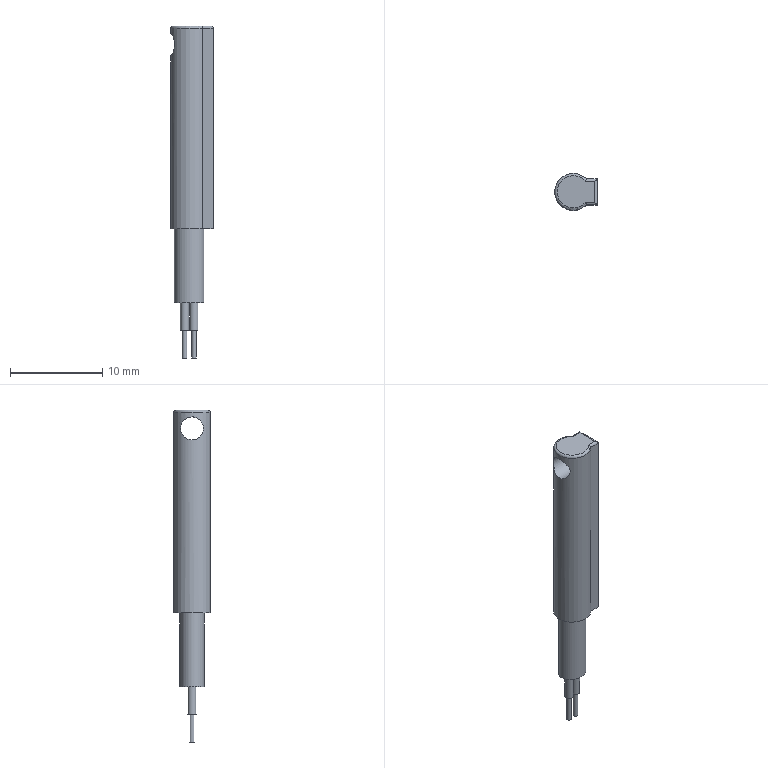Part | STEP file | ROTATION MC_NEW VER-0610_498 | 1 solid | 80 faces | box 4.6 x 4 x 36 mm | volume 360.691 mm3 | plane 44 | spline 26 | cylinder 9 | torus 1 | commonest cylinder face diameters 0.5 x5 0.9 x2 2.5 x1 4 x1